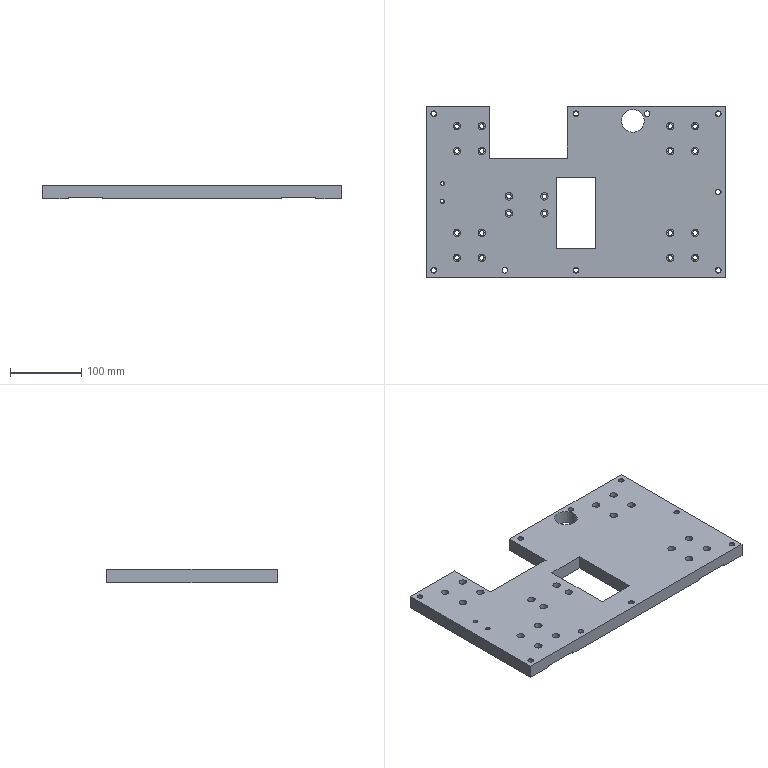Part | STEP file | Tube feed_id1014_x_t | 1 solid | 112 faces | box 420 x 240 x 19.3 mm | volume 1597092 mm3 | cylinder 52 | plane 42 | cone 18 | commonest cylinder face diameters 6.5 x20 10.5 x20 6.8 x7 5 x2 8 x2 32 x1